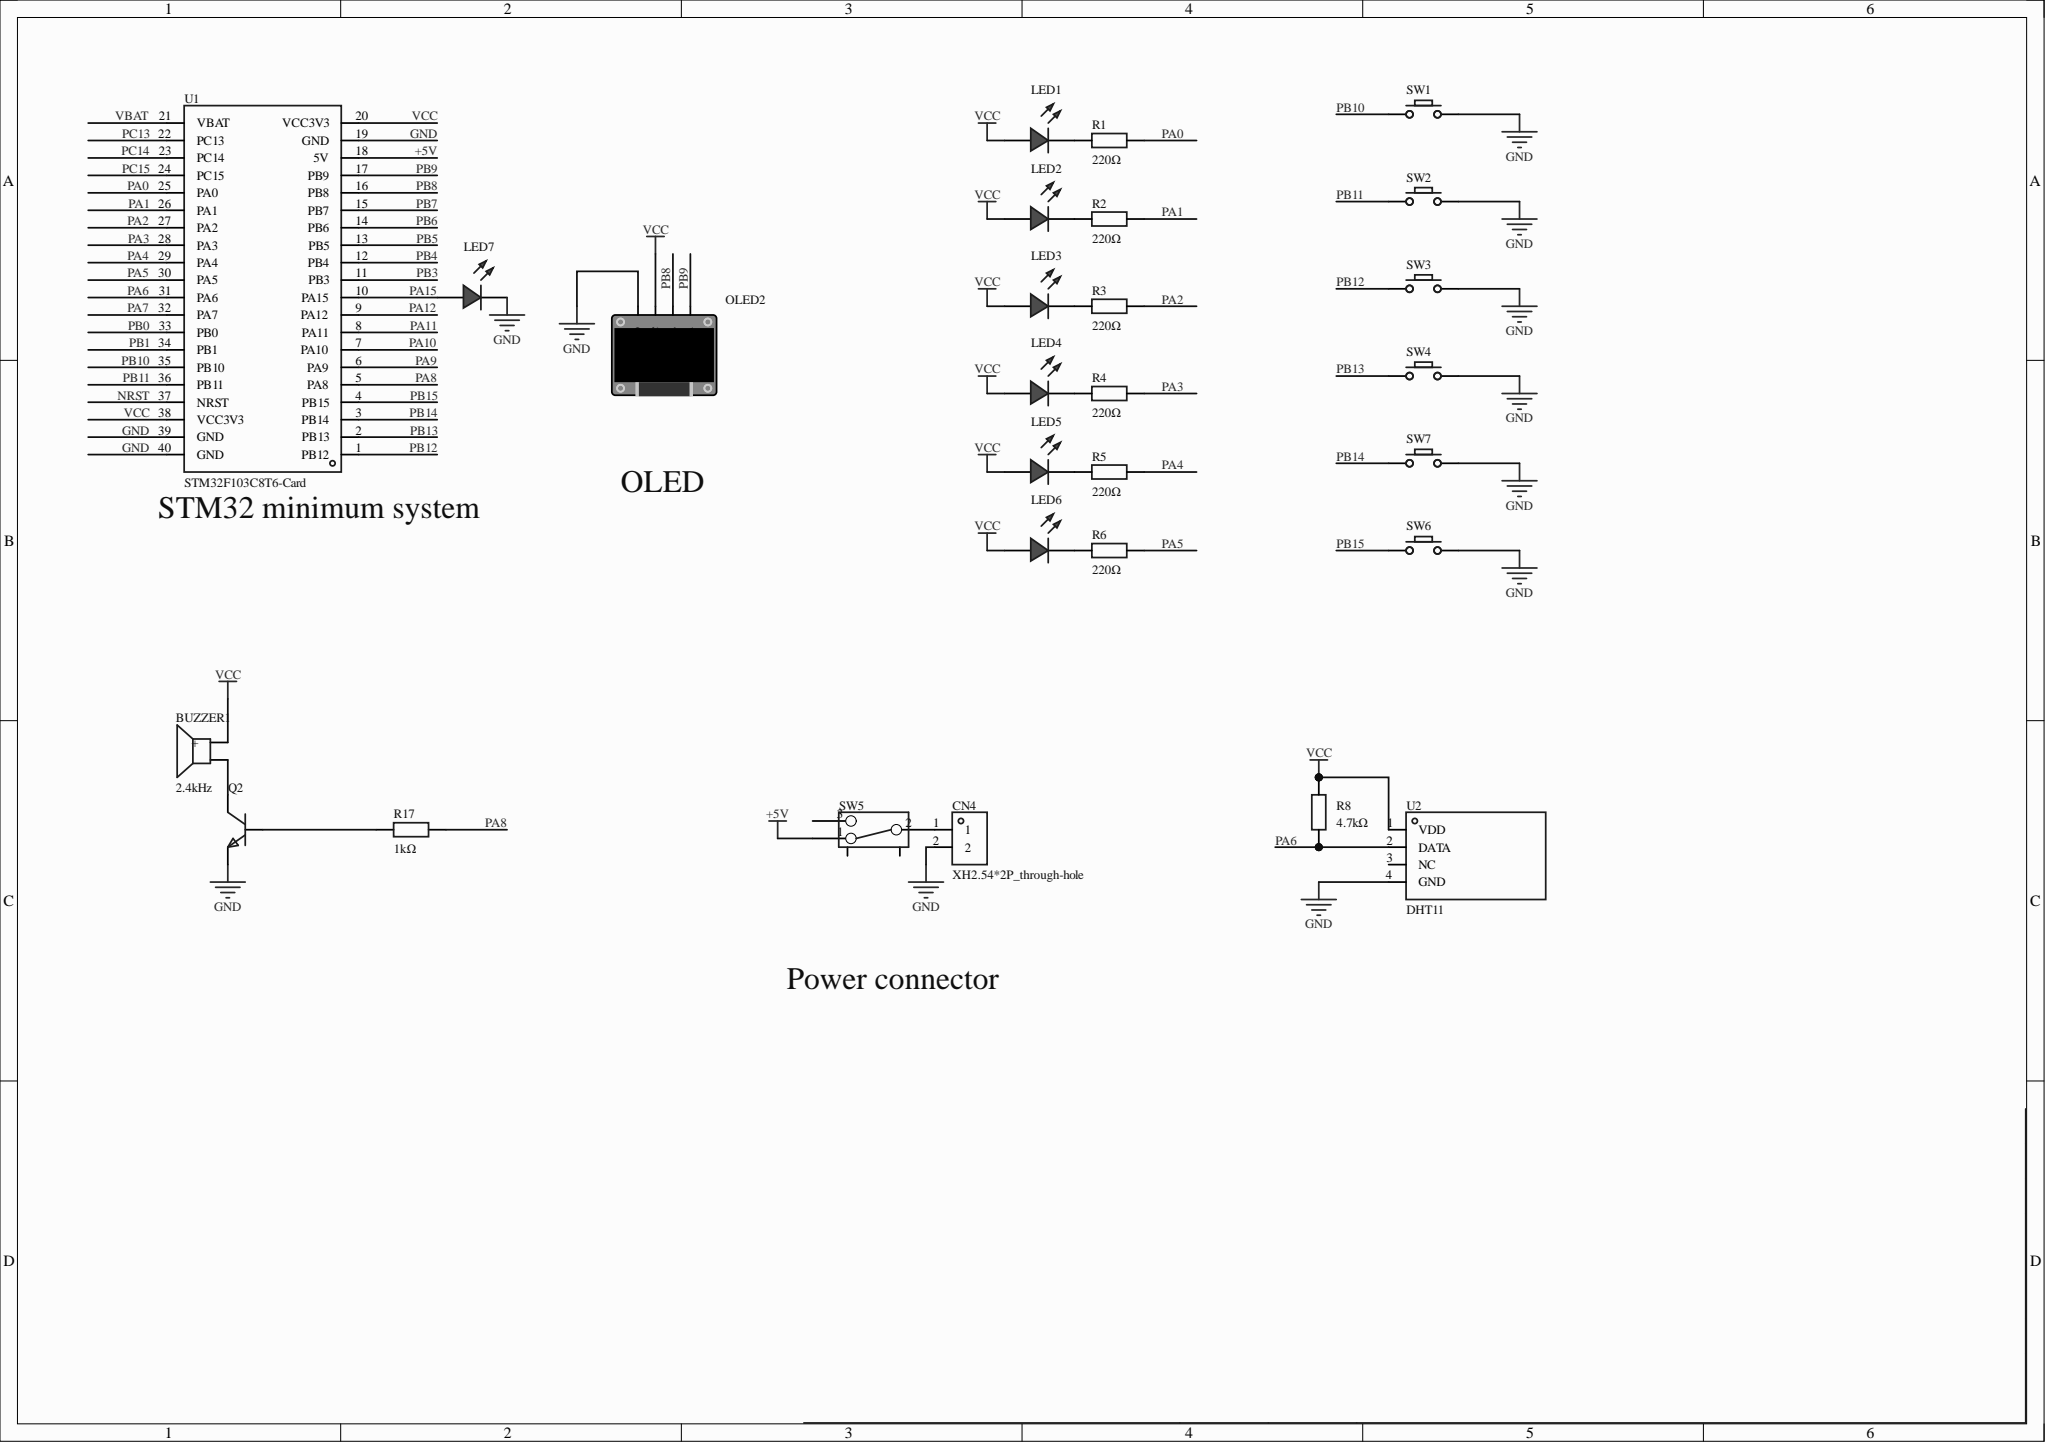Circuit board | Altium Designer | 28 parts | 29 nets
Bill of materials:
Comment,Description,Designator,Footprint,LibRef,Quantity
"2.4kHz","Driver mode: active (built-in driver circuit); construction type: electromagnetic; rated voltage: -; frequency: 2.4kHz; sound pressure (SPL): 85dB;","BUZZER1","BUZ-TH_BD12.0-P7.60-D0.6-FD","TMB12A05_C96093","1"
"XH2.54*2P_through-hole","","CN4","CONN-TH_2P-P2.50-XH2.54-2P","XH2.54*2P_直插","1"
"","","LED1, LED2, LED3, LED4, LED5, LED6, LED7","LED_TH-3mm","LED_TH-R_3mm","7"
"","","OLED2","0.96OLED_4P","0.96OLED模块_4P","1"
"","","Q2","S8050_TO_92","S8050_TO_NPN","1"
"220Ω","","R1, R2, R3, R4, R5, R6","Res_1/8W","Res_AXIAL-1/8W","6"
"4.7kΩ","","R8","Res_1/8W","Res_AXIAL-1/8W","1"
"1kΩ","Thick film resistor; resistance: 1kΩ; tolerance: ±1%; power: 100mW; working voltage: 75V; temperature coefficient: ±100ppm/?;","R17","R0603","RC0603FR-071KL","1"
"","","SW1, SW2, SW3, SW4, SW6, SW7","Key_TH_3.5x6x4.3","Key_TH_3.5x6x4.3","6"
"","","SW5","拨动开关","拨动开关_正","1"
"STM32F103C8T6-Card","","U1","CONN-TH_L53.3-W22.9_STM32F103C8T6-CARD","STM32F103C8T6-Card","1"
"DHT11","New capacitive digital temperature and humidity sensor; old model discontinued; 16.1x12.6x5.8mm","U2","SENSOR-TH_DHT11","DHT11","1"
Netlist (Protel format):
[
BUZZER1
BUZ-TH_BD12.0-P7.60-D0.6-FD
2.4kHz



]
[
CN4
CONN-TH_2P-P2.50-XH2.54-2P
XH2.54*2P_through-hole



]
[
LED1
LED_TH-3mm




]
[
LED2
LED_TH-3mm




]
[
LED3
LED_TH-3mm




]
[
LED4
LED_TH-3mm




]
[
LED5
LED_TH-3mm




]
[
LED6
LED_TH-3mm




]
[
LED7
LED_TH-3mm




]
[
OLED2
0.96OLED_4P




]
[
Q2
S8050_TO_92




]
[
R1
Res_1/8W
220Ω



]
[
R2
Res_1/8W
220Ω



]
[
R3
Res_1/8W
220Ω



]
[
R4
Res_1/8W
220Ω



]
[
R5
Res_1/8W
220Ω



]
[
R6
Res_1/8W
220Ω



]
[
R8
Res_1/8W
4.7kΩ



]
[
R17
R0603
1kΩ



]
[
SW1
Key_TH_3.5x6x4.3




]
[
SW2
Key_TH_3.5x6x4.3




]
[
SW3
Key_TH_3.5x6x4.3




]
[
SW4
Key_TH_3.5x6x4.3




]
[
SW5
拨动开关




]
[
SW6
Key_TH_3.5x6x4.3




]
[
SW7
Key_TH_3.5x6x4.3




]
[
U1
CONN-TH_L53.3-W22.9_STM32F103C8T6-CARD
STM32F103C8T6-Card



]
[
U2
SENSOR-TH_DHT11
DHT11



]
(
VCC
BUZZER1-1
LED1-1
LED2-1
LED3-1
LED4-1
LED5-1
LED6-1
OLED2-2
R8-2
U1-20
U1-38
U2-1
)
(
PB15
SW6-A
U1-4
)
(
PB14
SW7-A
U1-3
)
(
PB13
SW4-A
U1-2
)
(
PB12
SW3-A
U1-1
)
(
PB11
SW2-A
U1-36
)
(
PB10
SW1-A
U1-35
)
(
PB9
OLED2-4
U1-17
)
(
PB8
OLED2-3
U1-16
)
(
PA15
LED7-1
U1-10
)
(
PA8
R17-1
U1-5
)
(
PA6
R8-1
U1-31
U2-2
)
(
PA5
R6-2
U1-30
)
(
PA4
R5-2
U1-29
)
(
PA3
R4-2
U1-28
)
(
PA2
R3-2
U1-27
)
(
PA1
R2-2
U1-26
)
(
PA0
R1-2
U1-25
)
(
NetQ2_2
Q2-2
R17-2
)
(
NetLED6_2
LED6-2
R6-1
)
(
NetLED5_2
LED5-2
R5-1
)
(
NetLED4_2
LED4-2
R4-1
)
(
NetLED3_2
LED3-2
R3-1
)
(
NetLED2_2
LED2-2
R2-1
)
(
NetLED1_2
LED1-2
R1-1
)
(
NetCN4_1
CN4-1
SW5-2
)
(
NetBUZZER1_2
BUZZER1-2
Q2-3
)
(
GND
CN4-2
LED7-2
OLED2-1
Q2-1
SW1-B
SW2-B
SW3-B
SW4-B
SW6-B
SW7-B
U1-19
U1-39
U1-40
U2-4
)
(
+5V
SW5-1
U1-18
)